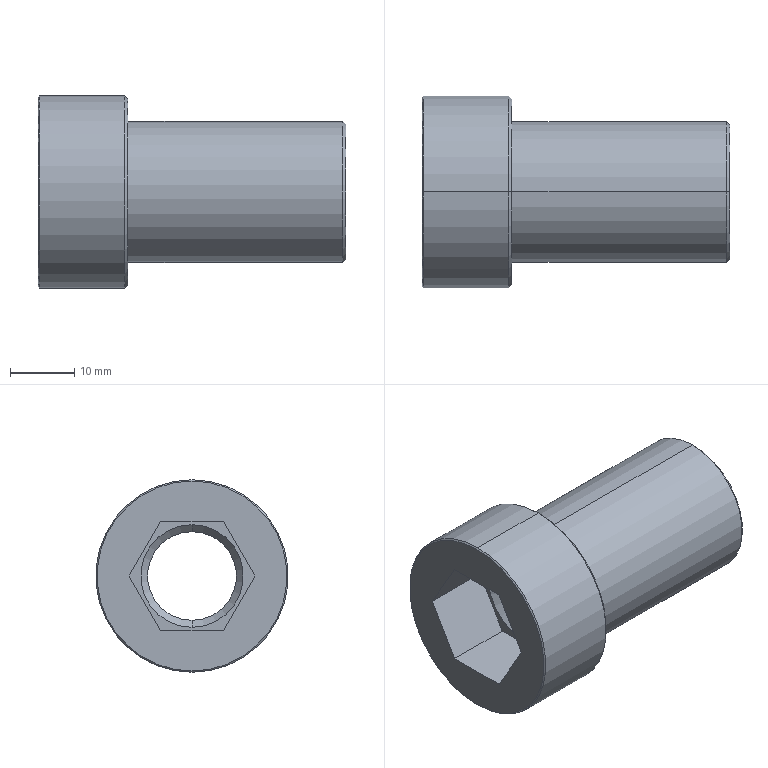Part | STEP file | SI160 | 1 solid | 26 faces | box 48 x 30 x 30 mm | volume 14480 mm3 | cone 10 | plane 10 | cylinder 6 | commonest cylinder face diameters 13.835 x2 22 x2 30 x2